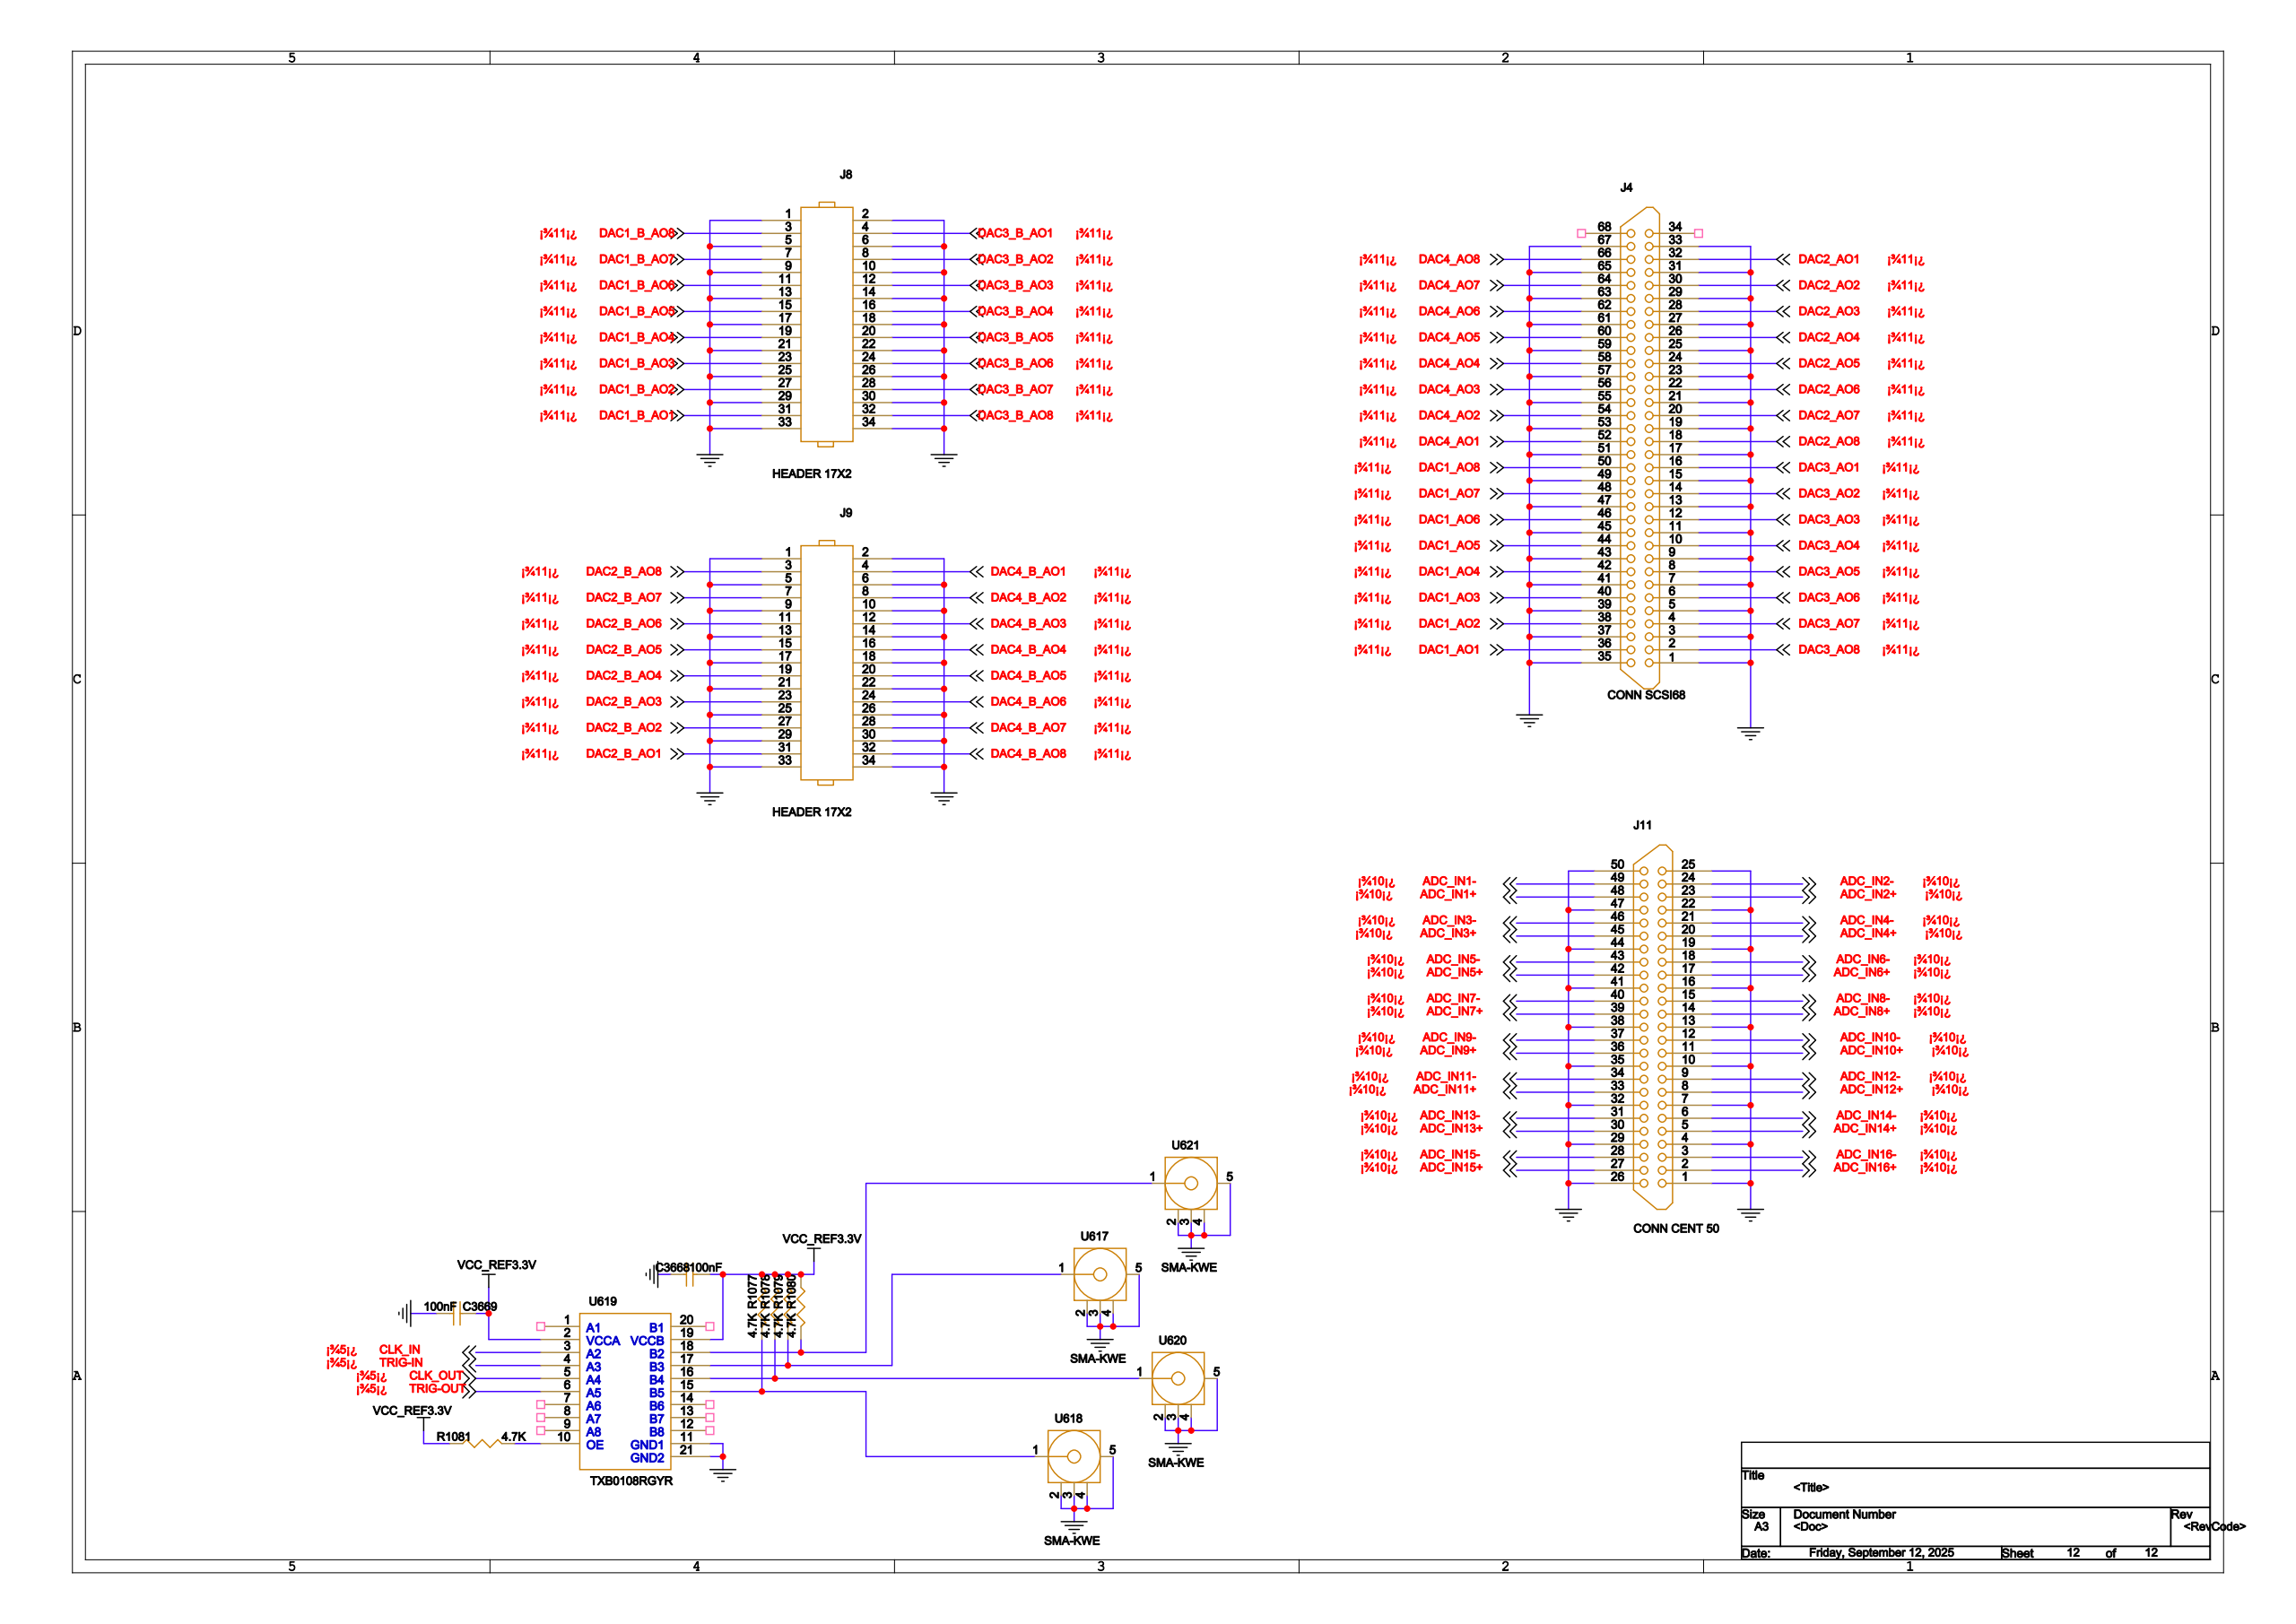Circuit board | Cadence Allegro | 528 parts | 530 nets | one sheet of the schematic
Parts on this sheet (reference | value | footprint):
C3669 | 100nF | C0402
J4 | CONN SCSI68 | SCSI68
J8 | HEADER 17X2 | CONN-TH_XH2_5-34P
J9 | HEADER 17X2 | CONN-TH_XH2_5-34P
J11 | CONN CENT 50 | SCSI50
R1077 | 4.7K | 0402
R1078 | 4.7K | 0402
R1079 | 4.7K | 0402
R1080 | 4.7K | 0402
R1081 | 4.7K | 0402
U617 | SMA-KWE | SMP-JHD_4_SMA_D5X5MM_SMA
U618 | SMA-KWE | SMP-JHD_4_SMA_D5X5MM_SMA
U619 | TXB0108RGYR | TXB0108RGYR
U620 | SMA-KWE | SMP-JHD_4_SMA_D5X5MM_SMA
U621 | SMA-KWE | SMP-JHD_4_SMA_D5X5MM_SMA
Nets of these parts (net: part-pin ...):
GND: C3669-2 U617-2 U617-3 U617-4 U617-5 U618-2 U618-3 U618-4 U618-5 U619-11 U619-21 U620-2 U620-3 U620-4 U620-5 U621-2 U621-3 U621-4 U621-5 J4-1 J4-3 J4-5 J4-7 J4-9 J4-11 J4-13 J4-15 J4-17 J4-19 J4-21 J4-23 J4-25 J4-27 J4-29 J4-31 J4-33 J4-35 J4-37 J4-39 J4-41 J4-43 J4-45 J4-47 J4-49 J4-51 J4-53 J4-55 J4-57 J4-59 J4-61 J4-63 J4-65 J4-67 J8-1 J8-2 J8-5 J8-6 J8-9 J8-10 J8-13 J8-14 J8-17 J8-18 J8-21 J8-22 J8-25 J8-26 J8-29 J8-30 J8-33 J8-34 J9-1 J9-2 J9-5 J9-6 J9-9 J9-10 J9-13 J9-14 J9-17 J9-18 J9-21 J9-22 J9-25 J9-26 J9-29 J9-30 J9-33 J9-34 J11-1 J11-4 J11-7 J11-10 J11-13 J11-16 J11-19 J11-22 J11-25 J11-26 J11-29 J11-32 J11-35 J11-38 J11-41 J11-44 J11-47 J11-50
VCC_REF3.3V: C3669-1 R1077-2 R1078-2 R1079-2 R1080-2 R1081-1 U619-2 U619-19
ADC_IN10+: J11-11
ADC_IN10-: J11-12
ADC_IN8+: J11-14
ADC_IN8-: J11-15
ADC_IN6+: J11-17
ADC_IN6-: J11-18
ADC_IN16+: J11-2
ADC_IN4+: J11-20
ADC_IN4-: J11-21
ADC_IN2+: J11-23
ADC_IN2-: J11-24
ADC_IN15+: J11-27
ADC_IN15-: J11-28
ADC_IN16-: J11-3
ADC_IN13+: J11-30
ADC_IN13-: J11-31
ADC_IN11+: J11-33
ADC_IN11-: J11-34
ADC_IN9+: J11-36
ADC_IN9-: J11-37
ADC_IN7+: J11-39
ADC_IN7-: J11-40
ADC_IN5+: J11-42
ADC_IN5-: J11-43
ADC_IN3+: J11-45
ADC_IN3-: J11-46
ADC_IN1+: J11-48
ADC_IN1-: J11-49
ADC_IN14+: J11-5
ADC_IN14-: J11-6
ADC_IN12+: J11-8
ADC_IN12-: J11-9
DAC1_B_AO6: J8-11
DAC3_B_AO3: J8-12
DAC1_B_AO5: J8-15
DAC3_B_AO4: J8-16
DAC1_B_AO4: J8-19
DAC3_B_AO5: J8-20
DAC1_B_AO3: J8-23
DAC3_B_AO6: J8-24
DAC1_B_AO2: J8-27
DAC3_B_AO7: J8-28
DAC1_B_AO8: J8-3
DAC1_B_AO1: J8-31
DAC3_B_AO8: J8-32
DAC3_B_AO1: J8-4
DAC1_B_AO7: J8-7
DAC3_B_AO2: J8-8
DAC2_B_AO6: J9-11
DAC4_B_AO3: J9-12
DAC2_B_AO5: J9-15
DAC4_B_AO4: J9-16
DAC2_B_AO4: J9-19
DAC4_B_AO5: J9-20
DAC2_B_AO3: J9-23
DAC4_B_AO6: J9-24
DAC2_B_AO2: J9-27
DAC4_B_AO7: J9-28
DAC2_B_AO8: J9-3
DAC2_B_AO1: J9-31
DAC4_B_AO8: J9-32
DAC4_B_AO1: J9-4
DAC2_B_AO7: J9-7
DAC4_B_AO2: J9-8
N18776267: R1077-1 U618-1 U619-15
N18989253: R1078-1 U619-16 U620-1
N18776575: R1079-1 U617-1 U619-17
N18989257: R1080-1 U619-18 U621-1
N18989334: R1081-2 U619-10
CLK_IN: U619-3
TRIG-IN: U619-4
CLK_OUT: U619-5
TRIG-OUT: U619-6
DAC3_AO4: J4-10
DAC3_AO3: J4-12
DAC3_AO2: J4-14
DAC3_AO1: J4-16
DAC2_AO8: J4-18
DAC3_AO8: J4-2
DAC2_AO7: J4-20
DAC2_AO6: J4-22
DAC2_AO5: J4-24
DAC2_AO4: J4-26
DAC2_AO3: J4-28
DAC2_AO2: J4-30
DAC2_AO1: J4-32
DAC1_AO1: J4-36
DAC1_AO2: J4-38
DAC3_AO7: J4-4
DAC1_AO3: J4-40
DAC1_AO4: J4-42
DAC1_AO5: J4-44
DAC1_AO6: J4-46
DAC1_AO7: J4-48
DAC1_AO8: J4-50
DAC4_AO1: J4-52
DAC4_AO2: J4-54
DAC4_AO3: J4-56
DAC4_AO4: J4-58
DAC3_AO6: J4-6
DAC4_AO5: J4-60
DAC4_AO6: J4-62
DAC4_AO7: J4-64
DAC4_AO8: J4-66
DAC3_AO5: J4-8